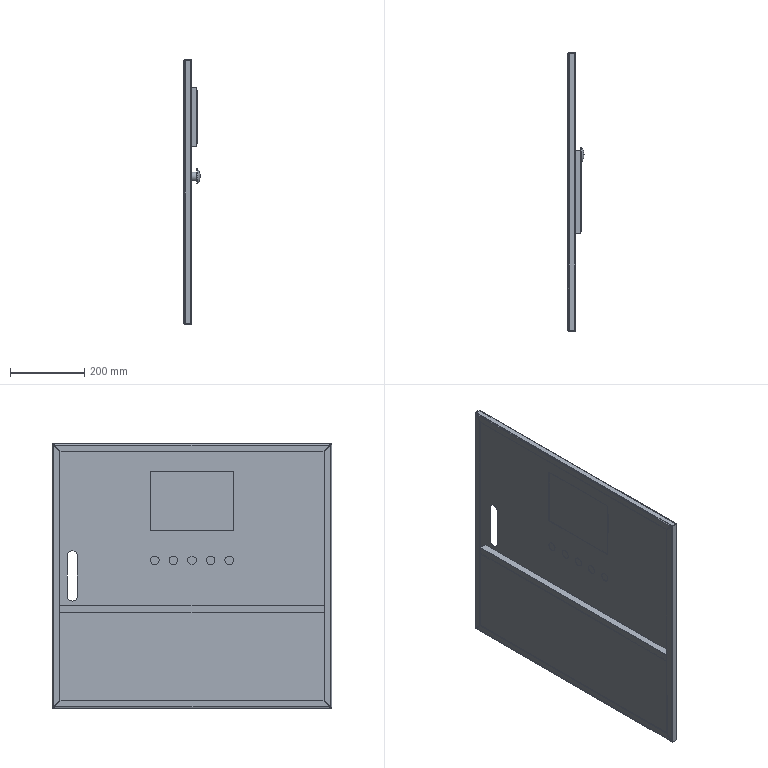Part | STEP file | PRT0544B-HK-005_B9T2-2 | 8 solids | 162 faces | box 43.5 x 750 x 710 mm | volume 1553231 mm3 | plane 87 | cylinder 65 | spline 8 | sphere 2 | commonest cylinder face diameters 23 x20 3 x8 5.2 x8 6 x8 27 x3 18.873 x2